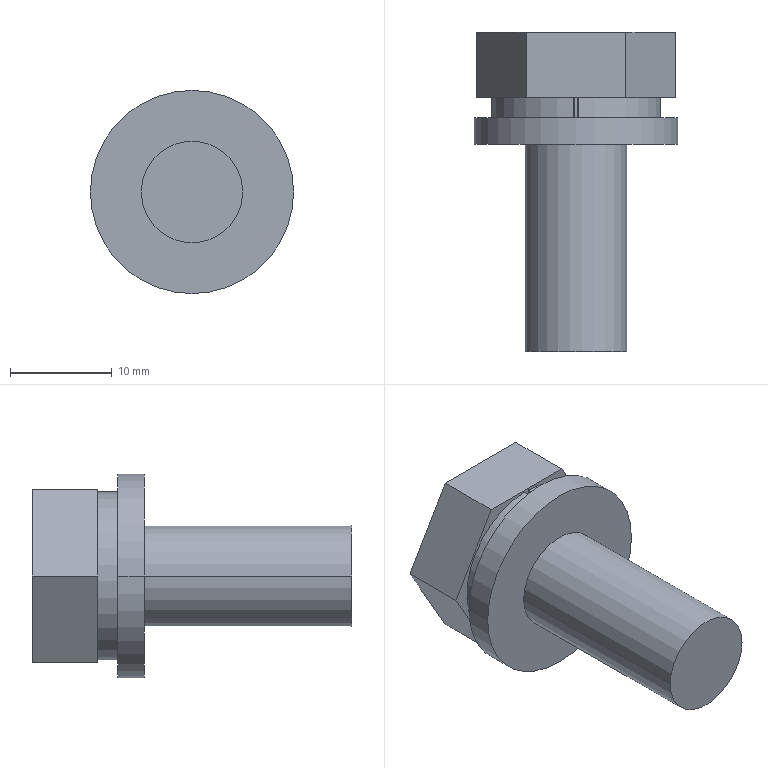Part | STEP file | LIB_68310857_M10X25 | 1 solid | 19 faces | box 20 x 31.4 x 20 mm | volume 4451 mm3 | plane 13 | cylinder 6 | commonest cylinder face diameters 10 x3 20 x2 16.6 x1
STEP:
#1=CARTESIAN_POINT('',(0.,0.,0.));
#2=DIRECTION('',(0.,0.,1.));
#3=DIRECTION('',(1.,0.,0.));
#4=AXIS2_PLACEMENT_3D('',#1,#2,#3);
#5=CARTESIAN_POINT('',(-4.907,0.,-8.5));
#6=VERTEX_POINT('',#5);
#7=CARTESIAN_POINT('',(-9.815,0.,0.));
#8=VERTEX_POINT('',#7);
#9=CARTESIAN_POINT('',(-4.907,0.,-8.5));
#10=DIRECTION('',(-0.5,0.,0.866));
#11=VECTOR('',#10,1.);
#12=LINE('',#9,#11);
#13=CARTESIAN_POINT('',(0.,0.,0.));
#14=DIRECTION('',(0.,1.,0.));
#15=DIRECTION('',(1.,0.,0.));
#16=AXIS2_PLACEMENT_3D('',#13,#14,#15);
#17=PLANE('',#16);
#18=CARTESIAN_POINT('',(-4.907,8.5));
#19=DIRECTION('',(-0.5,-0.866));
#20=VECTOR('',#19,1.);
#21=LINE('',#18,#20);
#22=(GEOMETRIC_REPRESENTATION_CONTEXT(2)PARAMETRIC_REPRESENTATION_CONTEXT()REPRESENTATION_CONTEXT('',''));
#23=DEFINITIONAL_REPRESENTATION('',(#21),#22);
#24=PCURVE('',#17,#23);
#25=CARTESIAN_POINT('',(-4.907,0.,-8.5));
#26=DIRECTION('',(-0.866,0.,-0.5));
#27=DIRECTION('',(-0.5,0.,0.866));
#28=AXIS2_PLACEMENT_3D('',#25,#26,#27);
#29=PLANE('',#28);
#30=CARTESIAN_POINT('',(0.,0.));
#31=DIRECTION('',(1.,0.));
#32=VECTOR('',#31,1.);
#33=LINE('',#30,#32);
#34=(GEOMETRIC_REPRESENTATION_CONTEXT(2)PARAMETRIC_REPRESENTATION_CONTEXT()REPRESENTATION_CONTEXT('',''));
#35=DEFINITIONAL_REPRESENTATION('',(#33),#34);
#36=PCURVE('',#29,#35);
#37=SURFACE_CURVE('',#12,(#24,#36),.PCURVE_S1.);
#38=EDGE_CURVE('',#6,#8,#37,.T.);
#39=ORIENTED_EDGE('',*,*,#38,.T.);
#40=CARTESIAN_POINT('',(-4.907,0.,8.5));
#41=VERTEX_POINT('',#40);
#42=CARTESIAN_POINT('',(-9.815,0.,0.));
#43=DIRECTION('',(0.5,0.,0.866));
#44=VECTOR('',#43,1.);
#45=LINE('',#42,#44);
#46=CARTESIAN_POINT('',(-9.815,0.));
#47=DIRECTION('',(0.5,-0.866));
#48=VECTOR('',#47,1.);
#49=LINE('',#46,#48);
#50=(GEOMETRIC_REPRESENTATION_CONTEXT(2)PARAMETRIC_REPRESENTATION_CONTEXT()REPRESENTATION_CONTEXT('',''));
#51=DEFINITIONAL_REPRESENTATION('',(#49),#50);
#52=PCURVE('',#17,#51);
#53=CARTESIAN_POINT('',(-9.815,0.,0.));
#54=DIRECTION('',(-0.866,0.,0.5));
#55=DIRECTION('',(0.5,0.,0.866));
#56=AXIS2_PLACEMENT_3D('',#53,#54,#55);
#57=PLANE('',#56);
#58=CARTESIAN_POINT('',(0.,0.));
#59=DIRECTION('',(1.,0.));
#60=VECTOR('',#59,1.);
#61=LINE('',#58,#60);
#62=(GEOMETRIC_REPRESENTATION_CONTEXT(2)PARAMETRIC_REPRESENTATION_CONTEXT()REPRESENTATION_CONTEXT('',''));
#63=DEFINITIONAL_REPRESENTATION('',(#61),#62);
#64=PCURVE('',#57,#63);
#65=SURFACE_CURVE('',#45,(#52,#64),.PCURVE_S1.);
#66=EDGE_CURVE('',#8,#41,#65,.T.);
#67=ORIENTED_EDGE('',*,*,#66,.T.);
#68=CARTESIAN_POINT('',(4.907,0.,8.5));
#69=VERTEX_POINT('',#68);
#70=CARTESIAN_POINT('',(-4.907,0.,8.5));
#71=DIRECTION('',(1.,0.,0.));
#72=VECTOR('',#71,1.);
#73=LINE('',#70,#72);
#74=CARTESIAN_POINT('',(-4.907,-8.5));
#75=DIRECTION('',(1.,0.));
#76=VECTOR('',#75,1.);
#77=LINE('',#74,#76);
#78=(GEOMETRIC_REPRESENTATION_CONTEXT(2)PARAMETRIC_REPRESENTATION_CONTEXT()REPRESENTATION_CONTEXT('',''));
#79=DEFINITIONAL_REPRESENTATION('',(#77),#78);
#80=PCURVE('',#17,#79);
#81=CARTESIAN_POINT('',(-4.907,0.,8.5));
#82=DIRECTION('',(0.,0.,1.));
#83=DIRECTION('',(1.,0.,0.));
#84=AXIS2_PLACEMENT_3D('',#81,#82,#83);
#85=PLANE('',#84);
#86=CARTESIAN_POINT('',(0.,0.));
#87=DIRECTION('',(1.,0.));
#88=VECTOR('',#87,1.);
#89=LINE('',#86,#88);
#90=(GEOMETRIC_REPRESENTATION_CONTEXT(2)PARAMETRIC_REPRESENTATION_CONTEXT()REPRESENTATION_CONTEXT('',''));
#91=DEFINITIONAL_REPRESENTATION('',(#89),#90);
#92=PCURVE('',#85,#91);
#93=SURFACE_CURVE('',#73,(#80,#92),.PCURVE_S1.);
#94=EDGE_CURVE('',#41,#69,#93,.T.);
#95=ORIENTED_EDGE('',*,*,#94,.T.);
#96=CARTESIAN_POINT('',(9.815,0.,0.));
#97=VERTEX_POINT('',#96);
#98=CARTESIAN_POINT('',(4.907,0.,8.5));
#99=DIRECTION('',(0.5,0.,-0.866));
#100=VECTOR('',#99,1.);
#101=LINE('',#98,#100);
#102=CARTESIAN_POINT('',(4.907,-8.5));
#103=DIRECTION('',(0.5,0.866));
#104=VECTOR('',#103,1.);
#105=LINE('',#102,#104);
#106=(GEOMETRIC_REPRESENTATION_CONTEXT(2)PARAMETRIC_REPRESENTATION_CONTEXT()REPRESENTATION_CONTEXT('',''));
#107=DEFINITIONAL_REPRESENTATION('',(#105),#106);
#108=PCURVE('',#17,#107);
#109=CARTESIAN_POINT('',(4.907,0.,8.5));
#110=DIRECTION('',(0.866,0.,0.5));
#111=DIRECTION('',(0.5,0.,-0.866));
#112=AXIS2_PLACEMENT_3D('',#109,#110,#111);
#113=PLANE('',#112);
#114=CARTESIAN_POINT('',(0.,0.));
#115=DIRECTION('',(1.,0.));
#116=VECTOR('',#115,1.);
#117=LINE('',#114,#116);
#118=(GEOMETRIC_REPRESENTATION_CONTEXT(2)PARAMETRIC_REPRESENTATION_CONTEXT()REPRESENTATION_CONTEXT('',''));
#119=DEFINITIONAL_REPRESENTATION('',(#117),#118);
#120=PCURVE('',#113,#119);
#121=SURFACE_CURVE('',#101,(#108,#120),.PCURVE_S1.);
#122=EDGE_CURVE('',#69,#97,#121,.T.);
#123=ORIENTED_EDGE('',*,*,#122,.T.);
#124=CARTESIAN_POINT('',(4.907,0.,-8.5));
#125=VERTEX_POINT('',#124);
#126=CARTESIAN_POINT('',(9.815,0.,0.));
#127=DIRECTION('',(-0.5,0.,-0.866));
#128=VECTOR('',#127,1.);
#129=LINE('',#126,#128);
#130=CARTESIAN_POINT('',(9.815,0.));
#131=DIRECTION('',(-0.5,0.866));
#132=VECTOR('',#131,1.);
#133=LINE('',#130,#132);
#134=(GEOMETRIC_REPRESENTATION_CONTEXT(2)PARAMETRIC_REPRESENTATION_CONTEXT()REPRESENTATION_CONTEXT('',''));
#135=DEFINITIONAL_REPRESENTATION('',(#133),#134);
#136=PCURVE('',#17,#135);
#137=CARTESIAN_POINT('',(9.815,0.,0.));
#138=DIRECTION('',(0.866,0.,-0.5));
#139=DIRECTION('',(-0.5,0.,-0.866));
#140=AXIS2_PLACEMENT_3D('',#137,#138,#139);
#141=PLANE('',#140);
#142=CARTESIAN_POINT('',(0.,0.));
#143=DIRECTION('',(1.,0.));
#144=VECTOR('',#143,1.);
#145=LINE('',#142,#144);
#146=(GEOMETRIC_REPRESENTATION_CONTEXT(2)PARAMETRIC_REPRESENTATION_CONTEXT()REPRESENTATION_CONTEXT('',''));
#147=DEFINITIONAL_REPRESENTATION('',(#145),#146);
#148=PCURVE('',#141,#147);
#149=SURFACE_CURVE('',#129,(#136,#148),.PCURVE_S1.);
#150=EDGE_CURVE('',#97,#125,#149,.T.);
#151=ORIENTED_EDGE('',*,*,#150,.T.);
#152=CARTESIAN_POINT('',(4.907,0.,-8.5));
#153=DIRECTION('',(-1.,0.,0.));
#154=VECTOR('',#153,1.);
#155=LINE('',#152,#154);
#156=CARTESIAN_POINT('',(4.907,8.5));
#157=DIRECTION('',(-1.,0.));
#158=VECTOR('',#157,1.);
#159=LINE('',#156,#158);
#160=(GEOMETRIC_REPRESENTATION_CONTEXT(2)PARAMETRIC_REPRESENTATION_CONTEXT()REPRESENTATION_CONTEXT('',''));
#161=DEFINITIONAL_REPRESENTATION('',(#159),#160);
#162=PCURVE('',#17,#161);
#163=CARTESIAN_POINT('',(4.907,0.,-8.5));
#164=DIRECTION('',(0.,0.,-1.));
#165=DIRECTION('',(-1.,0.,0.));
#166=AXIS2_PLACEMENT_3D('',#163,#164,#165);
#167=PLANE('',#166);
#168=CARTESIAN_POINT('',(0.,0.));
#169=DIRECTION('',(1.,0.));
#170=VECTOR('',#169,1.);
#171=LINE('',#168,#170);
#172=(GEOMETRIC_REPRESENTATION_CONTEXT(2)PARAMETRIC_REPRESENTATION_CONTEXT()REPRESENTATION_CONTEXT('',''));
#173=DEFINITIONAL_REPRESENTATION('',(#171),#172);
#174=PCURVE('',#167,#173);
#175=SURFACE_CURVE('',#155,(#162,#174),.PCURVE_S1.);
#176=EDGE_CURVE('',#125,#6,#175,.T.);
#177=ORIENTED_EDGE('',*,*,#176,.T.);
#178=EDGE_LOOP('',(#39,#67,#95,#123,#151,#177));
#179=FACE_BOUND('',#178,.F.);
#180=CARTESIAN_POINT('',(-0.25,0.,8.296));
#181=VERTEX_POINT('',#180);
#182=CARTESIAN_POINT('',(0.25,0.,8.296));
#183=VERTEX_POINT('',#182);
#184=CARTESIAN_POINT('',(0.,0.,0.));
#185=DIRECTION('',(0.,-1.,0.));
#186=DIRECTION('',(-0.03012,0.,0.9995));
#187=AXIS2_PLACEMENT_3D('',#184,#185,#186);
#188=CIRCLE('',#187,8.3);
#189=CARTESIAN_POINT('',(-0.25,-8.296));
#190=CARTESIAN_POINT('',(-14.619,-7.863));
#191=CARTESIAN_POINT('',(-7.06,4.365));
#192=CARTESIAN_POINT('',(0.5,16.592));
#193=CARTESIAN_POINT('',(7.31,3.932));
#194=CARTESIAN_POINT('',(14.119,-8.729));
#195=CARTESIAN_POINT('',(-0.25,-8.296));
#196=(BOUNDED_CURVE()B_SPLINE_CURVE(2,(#189,#190,#191,#192,#193,#194,#195),.UNSPECIFIED.,.T.,.F.)B_SPLINE_CURVE_WITH_KNOTS((1,2,2,2,2,1),(-2.094,0.,2.094,4.189,6.283,8.378),.UNSPECIFIED.)CURVE()GEOMETRIC_REPRESENTATION_ITEM()RATIONAL_B_SPLINE_CURVE((1.,0.5,1.,0.5,1.,0.5,1.))REPRESENTATION_ITEM(''));
#197=(GEOMETRIC_REPRESENTATION_CONTEXT(2)PARAMETRIC_REPRESENTATION_CONTEXT()REPRESENTATION_CONTEXT('',''));
#198=DEFINITIONAL_REPRESENTATION('',(#196),#197);
#199=PCURVE('',#17,#198);
#200=CARTESIAN_POINT('',(0.,0.,0.));
#201=DIRECTION('',(0.,-1.,0.));
#202=DIRECTION('',(0.,0.,-1.));
#203=AXIS2_PLACEMENT_3D('',#200,#201,#202);
#204=CYLINDRICAL_SURFACE('',#203,8.3);
#205=CARTESIAN_POINT('',(3.172,0.));
#206=DIRECTION('',(1.,0.));
#207=VECTOR('',#206,1.);
#208=LINE('',#205,#207);
#209=(GEOMETRIC_REPRESENTATION_CONTEXT(2)PARAMETRIC_REPRESENTATION_CONTEXT()REPRESENTATION_CONTEXT('',''));
#210=DEFINITIONAL_REPRESENTATION('',(#208),#209);
#211=PCURVE('',#204,#210);
#212=SURFACE_CURVE('',#188,(#199,#211),.PCURVE_S1.);
#213=EDGE_CURVE('',#181,#183,#212,.T.);
#214=ORIENTED_EDGE('',*,*,#213,.T.);
#215=CARTESIAN_POINT('',(0.1506,0.,4.998));
#216=VERTEX_POINT('',#215);
#217=CARTESIAN_POINT('',(0.25,0.,8.296));
#218=DIRECTION('',(-0.03012,0.,-0.9995));
#219=VECTOR('',#218,1.);
#220=LINE('',#217,#219);
#221=CARTESIAN_POINT('',(0.25,-8.296));
#222=DIRECTION('',(-0.03012,0.9995));
#223=VECTOR('',#222,1.);
#224=LINE('',#221,#223);
#225=(GEOMETRIC_REPRESENTATION_CONTEXT(2)PARAMETRIC_REPRESENTATION_CONTEXT()REPRESENTATION_CONTEXT('',''));
#226=DEFINITIONAL_REPRESENTATION('',(#224),#225);
#227=PCURVE('',#17,#226);
#228=CARTESIAN_POINT('',(0.25,0.,8.296));
#229=DIRECTION('',(-0.9995,0.,0.03012));
#230=DIRECTION('',(-0.03012,0.,-0.9995));
#231=AXIS2_PLACEMENT_3D('',#228,#229,#230);
#232=PLANE('',#231);
#233=CARTESIAN_POINT('',(0.,0.));
#234=DIRECTION('',(1.,0.));
#235=VECTOR('',#234,1.);
#236=LINE('',#233,#235);
#237=(GEOMETRIC_REPRESENTATION_CONTEXT(2)PARAMETRIC_REPRESENTATION_CONTEXT()REPRESENTATION_CONTEXT('',''));
#238=DEFINITIONAL_REPRESENTATION('',(#236),#237);
#239=PCURVE('',#232,#238);
#240=SURFACE_CURVE('',#220,(#227,#239),.PCURVE_S1.);
#241=EDGE_CURVE('',#183,#216,#240,.T.);
#242=ORIENTED_EDGE('',*,*,#241,.T.);
#243=CARTESIAN_POINT('',(-0.1506,0.,4.998));
#244=VERTEX_POINT('',#243);
#245=CARTESIAN_POINT('',(0.,0.,0.));
#246=DIRECTION('',(0.,-1.,0.));
#247=DIRECTION('',(0.03012,0.,0.9995));
#248=AXIS2_PLACEMENT_3D('',#245,#246,#247);
#249=CIRCLE('',#248,5.);
#250=CARTESIAN_POINT('',(0.1506,-4.998));
#251=CARTESIAN_POINT('',(-8.506,-5.259));
#252=CARTESIAN_POINT('',(-4.403,2.368));
#253=CARTESIAN_POINT('',(-0.3012,9.995));
#254=CARTESIAN_POINT('',(4.253,2.629));
#255=CARTESIAN_POINT('',(8.807,-4.737));
#256=CARTESIAN_POINT('',(0.1506,-4.998));
#257=(BOUNDED_CURVE()B_SPLINE_CURVE(2,(#250,#251,#252,#253,#254,#255,#256),.UNSPECIFIED.,.T.,.F.)B_SPLINE_CURVE_WITH_KNOTS((1,2,2,2,2,1),(-2.094,0.,2.094,4.189,6.283,8.378),.UNSPECIFIED.)CURVE()GEOMETRIC_REPRESENTATION_ITEM()RATIONAL_B_SPLINE_CURVE((1.,0.5,1.,0.5,1.,0.5,1.))REPRESENTATION_ITEM(''));
#258=(GEOMETRIC_REPRESENTATION_CONTEXT(2)PARAMETRIC_REPRESENTATION_CONTEXT()REPRESENTATION_CONTEXT('',''));
#259=DEFINITIONAL_REPRESENTATION('',(#257),#258);
#260=PCURVE('',#17,#259);
#261=CARTESIAN_POINT('',(0.,0.,0.));
#262=DIRECTION('',(0.,-1.,0.));
#263=DIRECTION('',(1.,0.,0.));
#264=AXIS2_PLACEMENT_3D('',#261,#262,#263);
#265=CYLINDRICAL_SURFACE('',#264,5.);
#266=CARTESIAN_POINT('',(1.541,0.));
#267=DIRECTION('',(1.,0.));
#268=VECTOR('',#267,1.);
#269=LINE('',#266,#268);
#270=(GEOMETRIC_REPRESENTATION_CONTEXT(2)PARAMETRIC_REPRESENTATION_CONTEXT()REPRESENTATION_CONTEXT('',''));
#271=DEFINITIONAL_REPRESENTATION('',(#269),#270);
#272=PCURVE('',#265,#271);
#273=SURFACE_CURVE('',#249,(#260,#272),.PCURVE_S1.);
#274=EDGE_CURVE('',#216,#244,#273,.T.);
#275=ORIENTED_EDGE('',*,*,#274,.T.);
#276=CARTESIAN_POINT('',(-0.1506,0.,4.998));
#277=DIRECTION('',(-0.03012,0.,0.9995));
#278=VECTOR('',#277,1.);
#279=LINE('',#276,#278);
#280=CARTESIAN_POINT('',(-0.1506,-4.998));
#281=DIRECTION('',(-0.03012,-0.9995));
#282=VECTOR('',#281,1.);
#283=LINE('',#280,#282);
#284=(GEOMETRIC_REPRESENTATION_CONTEXT(2)PARAMETRIC_REPRESENTATION_CONTEXT()REPRESENTATION_CONTEXT('',''));
#285=DEFINITIONAL_REPRESENTATION('',(#283),#284);
#286=PCURVE('',#17,#285);
#287=CARTESIAN_POINT('',(-0.1506,0.,4.998));
#288=DIRECTION('',(0.9995,0.,0.03012));
#289=DIRECTION('',(-0.03012,0.,0.9995));
#290=AXIS2_PLACEMENT_3D('',#287,#288,#289);
#291=PLANE('',#290);
#292=CARTESIAN_POINT('',(0.,0.));
#293=DIRECTION('',(1.,0.));
#294=VECTOR('',#293,1.);
#295=LINE('',#292,#294);
#296=(GEOMETRIC_REPRESENTATION_CONTEXT(2)PARAMETRIC_REPRESENTATION_CONTEXT()REPRESENTATION_CONTEXT('',''));
#297=DEFINITIONAL_REPRESENTATION('',(#295),#296);
#298=PCURVE('',#291,#297);
#299=SURFACE_CURVE('',#279,(#286,#298),.PCURVE_S1.);
#300=EDGE_CURVE('',#244,#181,#299,.T.);
#301=ORIENTED_EDGE('',*,*,#300,.T.);
#302=EDGE_LOOP('',(#214,#242,#275,#301));
#303=FACE_BOUND('',#302,.F.);
#304=ADVANCED_FACE('',(#179,#303),#17,.F.);
#305=ORIENTED_EDGE('',*,*,#38,.F.);
#306=CARTESIAN_POINT('',(-4.907,6.4,-8.5));
#307=VERTEX_POINT('',#306);
#308=CARTESIAN_POINT('',(-4.907,0.,-8.5));
#309=DIRECTION('',(0.,1.,0.));
#310=VECTOR('',#309,1.);
#311=LINE('',#308,#310);
#312=CARTESIAN_POINT('',(0.,0.));
#313=DIRECTION('',(0.,1.));
#314=VECTOR('',#313,1.);
#315=LINE('',#312,#314);
#316=(GEOMETRIC_REPRESENTATION_CONTEXT(2)PARAMETRIC_REPRESENTATION_CONTEXT()REPRESENTATION_CONTEXT('',''));
#317=DEFINITIONAL_REPRESENTATION('',(#315),#316);
#318=PCURVE('',#29,#317);
#319=CARTESIAN_POINT('',(9.815,0.));
#320=DIRECTION('',(0.,1.));
#321=VECTOR('',#320,1.);
#322=LINE('',#319,#321);
#323=(GEOMETRIC_REPRESENTATION_CONTEXT(2)PARAMETRIC_REPRESENTATION_CONTEXT()REPRESENTATION_CONTEXT('',''));
#324=DEFINITIONAL_REPRESENTATION('',(#322),#323);
#325=PCURVE('',#167,#324);
#326=SURFACE_CURVE('',#311,(#318,#325),.PCURVE_S1.);
#327=EDGE_CURVE('',#6,#307,#326,.T.);
#328=ORIENTED_EDGE('',*,*,#327,.T.);
#329=CARTESIAN_POINT('',(-9.815,6.4,0.));
#330=VERTEX_POINT('',#329);
#331=CARTESIAN_POINT('',(-4.907,6.4,-8.5));
#332=DIRECTION('',(-0.5,0.,0.866));
#333=VECTOR('',#332,1.);
#334=LINE('',#331,#333);
#335=CARTESIAN_POINT('',(0.,6.4));
#336=DIRECTION('',(1.,0.));
#337=VECTOR('',#336,1.);
#338=LINE('',#335,#337);
#339=(GEOMETRIC_REPRESENTATION_CONTEXT(2)PARAMETRIC_REPRESENTATION_CONTEXT()REPRESENTATION_CONTEXT('',''));
#340=DEFINITIONAL_REPRESENTATION('',(#338),#339);
#341=PCURVE('',#29,#340);
#342=CARTESIAN_POINT('',(0.,6.4,0.));
#343=DIRECTION('',(0.,1.,0.));
#344=DIRECTION('',(1.,0.,0.));
#345=AXIS2_PLACEMENT_3D('',#342,#343,#344);
#346=PLANE('',#345);
#347=CARTESIAN_POINT('',(-4.907,8.5));
#348=DIRECTION('',(-0.5,-0.866));
#349=VECTOR('',#348,1.);
#350=LINE('',#347,#349);
#351=(GEOMETRIC_REPRESENTATION_CONTEXT(2)PARAMETRIC_REPRESENTATION_CONTEXT()REPRESENTATION_CONTEXT('',''));
#352=DEFINITIONAL_REPRESENTATION('',(#350),#351);
#353=PCURVE('',#346,#352);
#354=SURFACE_CURVE('',#334,(#341,#353),.PCURVE_S1.);
#355=EDGE_CURVE('',#307,#330,#354,.T.);
#356=ORIENTED_EDGE('',*,*,#355,.T.);
#357=CARTESIAN_POINT('',(-9.815,0.,0.));
#358=DIRECTION('',(0.,1.,0.));
#359=VECTOR('',#358,1.);
#360=LINE('',#357,#359);
#361=CARTESIAN_POINT('',(9.815,0.));
#362=DIRECTION('',(0.,1.));
#363=VECTOR('',#362,1.);
#364=LINE('',#361,#363);
#365=(GEOMETRIC_REPRESENTATION_CONTEXT(2)PARAMETRIC_REPRESENTATION_CONTEXT()REPRESENTATION_CONTEXT('',''));
#366=DEFINITIONAL_REPRESENTATION('',(#364),#365);
#367=PCURVE('',#29,#366);
#368=CARTESIAN_POINT('',(0.,0.));
#369=DIRECTION('',(0.,1.));
#370=VECTOR('',#369,1.);
#371=LINE('',#368,#370);
#372=(GEOMETRIC_REPRESENTATION_CONTEXT(2)PARAMETRIC_REPRESENTATION_CONTEXT()REPRESENTATION_CONTEXT('',''));
#373=DEFINITIONAL_REPRESENTATION('',(#371),#372);
#374=PCURVE('',#57,#373);
#375=SURFACE_CURVE('',#360,(#367,#374),.PCURVE_S1.);
#376=EDGE_CURVE('',#8,#330,#375,.T.);
#377=ORIENTED_EDGE('',*,*,#376,.F.);
#378=EDGE_LOOP('',(#305,#328,#356,#377));
#379=FACE_BOUND('',#378,.F.);
#380=ADVANCED_FACE('',(#379),#29,.T.);
#381=ORIENTED_EDGE('',*,*,#176,.F.);
#382=CARTESIAN_POINT('',(4.907,6.4,-8.5));
#383=VERTEX_POINT('',#382);
#384=CARTESIAN_POINT('',(4.907,0.,-8.5));
#385=DIRECTION('',(0.,1.,0.));
#386=VECTOR('',#385,1.);
#387=LINE('',#384,#386);
#388=CARTESIAN_POINT('',(0.,0.));
#389=DIRECTION('',(0.,1.));
#390=VECTOR('',#389,1.);
#391=LINE('',#388,#390);
#392=(GEOMETRIC_REPRESENTATION_CONTEXT(2)PARAMETRIC_REPRESENTATION_CONTEXT()REPRESENTATION_CONTEXT('',''));
#393=DEFINITIONAL_REPRESENTATION('',(#391),#392);
#394=PCURVE('',#167,#393);
#395=CARTESIAN_POINT('',(9.815,0.));
#396=DIRECTION('',(0.,1.));
#397=VECTOR('',#396,1.);
#398=LINE('',#395,#397);
#399=(GEOMETRIC_REPRESENTATION_CONTEXT(2)PARAMETRIC_REPRESENTATION_CONTEXT()REPRESENTATION_CONTEXT('',''));
#400=DEFINITIONAL_REPRESENTATION('',(#398),#399);
#401=PCURVE('',#141,#400);
#402=SURFACE_CURVE('',#387,(#394,#401),.PCURVE_S1.);
#403=EDGE_CURVE('',#125,#383,#402,.T.);
#404=ORIENTED_EDGE('',*,*,#403,.T.);
#405=CARTESIAN_POINT('',(4.907,6.4,-8.5));
#406=DIRECTION('',(-1.,0.,0.));
#407=VECTOR('',#406,1.);
#408=LINE('',#405,#407);
#409=CARTESIAN_POINT('',(0.,6.4));
#410=DIRECTION('',(1.,0.));
#411=VECTOR('',#410,1.);
#412=LINE('',#409,#411);
#413=(GEOMETRIC_REPRESENTATION_CONTEXT(2)PARAMETRIC_REPRESENTATION_CONTEXT()REPRESENTATION_CONTEXT('',''));
#414=DEFINITIONAL_REPRESENTATION('',(#412),#413);
#415=PCURVE('',#167,#414);
#416=CARTESIAN_POINT('',(4.907,8.5));
#417=DIRECTION('',(-1.,0.));
#418=VECTOR('',#417,1.);
#419=LINE('',#416,#418);
#420=(GEOMETRIC_REPRESENTATION_CONTEXT(2)PARAMETRIC_REPRESENTATION_CONTEXT()REPRESENTATION_CONTEXT('',''));
#421=DEFINITIONAL_REPRESENTATION('',(#419),#420);
#422=PCURVE('',#346,#421);
#423=SURFACE_CURVE('',#408,(#415,#422),.PCURVE_S1.);
#424=EDGE_CURVE('',#383,#307,#423,.T.);
#425=ORIENTED_EDGE('',*,*,#424,.T.);
#426=ORIENTED_EDGE('',*,*,#327,.F.);
#427=EDGE_LOOP('',(#381,#404,#425,#426));
#428=FACE_BOUND('',#427,.F.);
#429=ADVANCED_FACE('',(#428),#167,.T.);
#430=ORIENTED_EDGE('',*,*,#150,.F.);
#431=CARTESIAN_POINT('',(9.815,6.4,0.));
#432=VERTEX_POINT('',#431);
#433=CARTESIAN_POINT('',(9.815,0.,0.));
#434=DIRECTION('',(0.,1.,0.));
#435=VECTOR('',#434,1.);
#436=LINE('',#433,#435);
#437=CARTESIAN_POINT('',(0.,0.));
#438=DIRECTION('',(0.,1.));
#439=VECTOR('',#438,1.);
#440=LINE('',#437,#439);
#441=(GEOMETRIC_REPRESENTATION_CONTEXT(2)PARAMETRIC_REPRESENTATION_CONTEXT()REPRESENTATION_CONTEXT('',''));
#442=DEFINITIONAL_REPRESENTATION('',(#440),#441);
#443=PCURVE('',#141,#442);
#444=CARTESIAN_POINT('',(9.815,0.));
#445=DIRECTION('',(0.,1.));
#446=VECTOR('',#445,1.);
#447=LINE('',#444,#446);
#448=(GEOMETRIC_REPRESENTATION_CONTEXT(2)PARAMETRIC_REPRESENTATION_CONTEXT()REPRESENTATION_CONTEXT('',''));
#449=DEFINITIONAL_REPRESENTATION('',(#447),#448);
#450=PCURVE('',#113,#449);
#451=SURFACE_CURVE('',#436,(#443,#450),.PCURVE_S1.);
#452=EDGE_CURVE('',#97,#432,#451,.T.);
#453=ORIENTED_EDGE('',*,*,#452,.T.);
#454=CARTESIAN_POINT('',(9.815,6.4,0.));
#455=DIRECTION('',(-0.5,0.,-0.866));
#456=VECTOR('',#455,1.);
#457=LINE('',#454,#456);
#458=CARTESIAN_POINT('',(0.,6.4));
#459=DIRECTION('',(1.,0.));
#460=VECTOR('',#459,1.);
#461=LINE('',#458,#460);
#462=(GEOMETRIC_REPRESENTATION_CONTEXT(2)PARAMETRIC_REPRESENTATION_CONTEXT()REPRESENTATION_CONTEXT('',''));
#463=DEFINITIONAL_REPRESENTATION('',(#461),#462);
#464=PCURVE('',#141,#463);
#465=CARTESIAN_POINT('',(9.815,0.));
#466=DIRECTION('',(-0.5,0.866));
#467=VECTOR('',#466,1.);
#468=LINE('',#465,#467);
#469=(GEOMETRIC_REPRESENTATION_CONTEXT(2)PARAMETRIC_REPRESENTATION_CONTEXT()REPRESENTATION_CONTEXT('',''));
#470=DEFINITIONAL_REPRESENTATION('',(#468),#469);
#471=PCURVE('',#346,#470);
#472=SURFACE_CURVE('',#457,(#464,#471),.PCURVE_S1.);
#473=EDGE_CURVE('',#432,#383,#472,.T.);
#474=ORIENTED_EDGE('',*,*,#473,.T.);
#475=ORIENTED_EDGE('',*,*,#403,.F.);
#476=EDGE_LOOP('',(#430,#453,#474,#475));
#477=FACE_BOUND('',#476,.F.);
#478=ADVANCED_FACE('',(#477),#141,.T.);
#479=ORIENTED_EDGE('',*,*,#122,.F.);
#480=CARTESIAN_POINT('',(4.907,6.4,8.5));
#481=VERTEX_POINT('',#480);
#482=CARTESIAN_POINT('',(4.907,0.,8.5));
#483=DIRECTION('',(0.,1.,0.));
#484=VECTOR('',#483,1.);
#485=LINE('',#482,#484);
#486=CARTESIAN_POINT('',(0.,0.));
#487=DIRECTION('',(0.,1.));
#488=VECTOR('',#487,1.);
#489=LINE('',#486,#488);
#490=(GEOMETRIC_REPRESENTATION_CONTEXT(2)PARAMETRIC_REPRESENTATION_CONTEXT()REPRESENTATION_CONTEXT('',''));
#491=DEFINITIONAL_REPRESENTATION('',(#489),#490);
#492=PCURVE('',#113,#491);
#493=CARTESIAN_POINT('',(9.815,0.));
#494=DIRECTION('',(0.,1.));
#495=VECTOR('',#494,1.);
#496=LINE('',#493,#495);
#497=(GEOMETRIC_REPRESENTATION_CONTEXT(2)PARAMETRIC_REPRESENTATION_CONTEXT()REPRESENTATION_CONTEXT('',''));
#498=DEFINITIONAL_REPRESENTATION('',(#496),#497);
#499=PCURVE('',#85,#498);
#500=SURFACE_CURVE('',#485,(#492,#499),.PCURVE_S1.);
#501=EDGE_CURVE('',#69,#481,#500,.T.);
#502=ORIENTED_EDGE('',*,*,#501,.T.);
#503=CARTESIAN_POINT('',(4.907,6.4,8.5));
#504=DIRECTION('',(0.5,0.,-0.866));
#505=VECTOR('',#504,1.);
#506=LINE('',#503,#505);
#507=CARTESIAN_POINT('',(0.,6.4));
#508=DIRECTION('',(1.,0.));
#509=VECTOR('',#508,1.);
#510=LINE('',#507,#509);
#511=(GEOMETRIC_REPRESENTATION_CONTEXT(2)PARAMETRIC_REPRESENTATION_CONTEXT()REPRESENTATION_CONTEXT('',''));
#512=DEFINITIONAL_REPRESENTATION('',(#510),#511);
#513=PCURVE('',#113,#512);
#514=CARTESIAN_POINT('',(4.907,-8.5));
#515=DIRECTION('',(0.5,0.866));
#516=VECTOR('',#515,1.);
#517=LINE('',#514,#516);
#518=(GEOMETRIC_REPRESENTATION_CONTEXT(2)PARAMETRIC_REPRESENTATION_CONTEXT()REPRESENTATION_CONTEXT('',''));
#519=DEFINITIONAL_REPRESENTATION('',(#517),#518);
#520=PCURVE('',#346,#519);
#521=SURFACE_CURVE('',#506,(#513,#520),.PCURVE_S1.);
#522=EDGE_CURVE('',#481,#432,#521,.T.);
#523=ORIENTED_EDGE('',*,*,#522,.T.);
#524=ORIENTED_EDGE('',*,*,#452,.F.);
#525=EDGE_LOOP('',(#479,#502,#523,#524));
#526=FACE_BOUND('',#525,.F.);
#527=ADVANCED_FACE('',(#526),#113,.T.);
#528=ORIENTED_EDGE('',*,*,#94,.F.);
#529=CARTESIAN_POINT('',(-4.907,6.4,8.5));
#530=VERTEX_POINT('',#529);
#531=CARTESIAN_POINT('',(-4.907,0.,8.5));
#532=DIRECTION('',(0.,1.,0.));
#533=VECTOR('',#532,1.);
#534=LINE('',#531,#533);
#535=CARTESIAN_POINT('',(0.,0.));
#536=DIRECTION('',(0.,1.));
#537=VECTOR('',#536,1.);
#538=LINE('',#535,#537);
#539=(GEOMETRIC_REPRESENTATION_CONTEXT(2)PARAMETRIC_REPRESENTATION_CONTEXT()REPRESENTATION_CONTEXT('',''));
#540=DEFINITIONAL_REPRESENTATION('',(#538),#539);
#541=PCURVE('',#85,#540);
#542=CARTESIAN_POINT('',(9.815,0.));
#543=DIRECTION('',(0.,1.));
#544=VECTOR('',#543,1.);
#545=LINE('',#542,#544);
#546=(GEOMETRIC_REPRESENTATION_CONTEXT(2)PARAMETRIC_REPRESENTATION_CONTEXT()REPRESENTATION_CONTEXT('',''));
#547=DEFINITIONAL_REPRESENTATION('',(#545),#546);
#548=PCURVE('',#57,#547);
#549=SURFACE_CURVE('',#534,(#541,#548),.PCURVE_S1.);
#550=EDGE_CURVE('',#41,#530,#549,.T.);
#551=ORIENTED_EDGE('',*,*,#550,.T.);
#552=CARTESIAN_POINT('',(-4.907,6.4,8.5));
#553=DIRECTION('',(1.,0.,0.));
#554=VECTOR('',#553,1.);
#555=LINE('',#552,#554);
#556=CARTESIAN_POINT('',(0.,6.4));
#557=DIRECTION('',(1.,0.));
#558=VECTOR('',#557,1.);
#559=LINE('',#556,#558);
#560=(GEOMETRIC_REPRESENTATION_CONTEXT(2)PARAMETRIC_REPRESENTATION_CONTEXT()REPRESENTATION_CONTEXT('',''));
#561=DEFINITIONAL_REPRESENTATION('',(#559),#560);
#562=PCURVE('',#85,#561);
#563=CARTESIAN_POINT('',(-4.907,-8.5));
#564=DIRECTION('',(1.,0.));
#565=VECTOR('',#564,1.);
#566=LINE('',#563,#565);
#567=(GEOMETRIC_REPRESENTATION_CONTEXT(2)PARAMETRIC_REPRESENTATION_CONTEXT()REPRESENTATION_CONTEXT('',''));
#568=DEFINITIONAL_REPRESENTATION('',(#566),#567);
#569=PCURVE('',#346,#568);
#570=SURFACE_CURVE('',#555,(#562,#569),.PCURVE_S1.);
#571=EDGE_CURVE('',#530,#481,#570,.T.);
#572=ORIENTED_EDGE('',*,*,#571,.T.);
#573=ORIENTED_EDGE('',*,*,#501,.F.);
#574=EDGE_LOOP('',(#528,#551,#572,#573));
#575=FACE_BOUND('',#574,.F.);
#576=ADVANCED_FACE('',(#575),#85,.T.);
#577=ORIENTED_EDGE('',*,*,#66,.F.);
#578=ORIENTED_EDGE('',*,*,#376,.T.);
#579=CARTESIAN_POINT('',(-9.815,6.4,0.));
#580=DIRECTION('',(0.5,0.,0.866));
#581=VECTOR('',#580,1.);
#582=LINE('',#579,#581);
#583=CARTESIAN_POINT('',(0.,6.4));
#584=DIRECTION('',(1.,0.));
#585=VECTOR('',#584,1.);
#586=LINE('',#583,#585);
#587=(GEOMETRIC_REPRESENTATION_CONTEXT(2)PARAMETRIC_REPRESENTATION_CONTEXT()REPRESENTATION_CONTEXT('',''));
#588=DEFINITIONAL_REPRESENTATION('',(#586),#587);
#589=PCURVE('',#57,#588);
#590=CARTESIAN_POINT('',(-9.815,0.));
#591=DIRECTION('',(0.5,-0.866));
#592=VECTOR('',#591,1.);
#593=LINE('',#590,#592);
#594=(GEOMETRIC_REPRESENTATION_CONTEXT(2)PARAMETRIC_REPRESENTATION_CONTEXT()REPRESENTATION_CONTEXT('',''));
#595=DEFINITIONAL_REPRESENTATION('',(#593),#594);
#596=PCURVE('',#346,#595);
#597=SURFACE_CURVE('',#582,(#589,#596),.PCURVE_S1.);
#598=EDGE_CURVE('',#330,#530,#597,.T.);
#599=ORIENTED_EDGE('',*,*,#598,.T.);
#600=ORIENTED_EDGE('',*,*,#550,.F.);
#601=EDGE_LOOP('',(#577,#578,#599,#600));
#602=FACE_BOUND('',#601,.F.);
#603=ADVANCED_FACE('',(#602),#57,.T.);
#604=ORIENTED_EDGE('',*,*,#355,.F.);
#605=ORIENTED_EDGE('',*,*,#424,.F.);
#606=ORIENTED_EDGE('',*,*,#473,.F.);
#607=ORIENTED_EDGE('',*,*,#522,.F.);
#608=ORIENTED_EDGE('',*,*,#571,.F.);
#609=ORIENTED_EDGE('',*,*,#598,.F.);
#610=EDGE_LOOP('',(#604,#605,#606,#607,#608,#609));
#611=FACE_BOUND('',#610,.F.);
#612=ADVANCED_FACE('',(#611),#346,.T.);
#613=CARTESIAN_POINT('',(-0.25,-2.,8.296));
#614=VERTEX_POINT('',#613);
#615=CARTESIAN_POINT('',(-0.25,0.,8.296));
#616=DIRECTION('',(0.,-1.,0.));
#617=VECTOR('',#616,1.);
#618=LINE('',#615,#617);
#619=CARTESIAN_POINT('',(3.172,0.));
#620=DIRECTION('',(0.,1.));
#621=VECTOR('',#620,1.);
#622=LINE('',#619,#621);
#623=(GEOMETRIC_REPRESENTATION_CONTEXT(2)PARAMETRIC_REPRESENTATION_CONTEXT()REPRESENTATION_CONTEXT('',''));
#624=DEFINITIONAL_REPRESENTATION('',(#622),#623);
#625=PCURVE('',#204,#624);
#626=CARTESIAN_POINT('',(3.3,0.));
#627=DIRECTION('',(0.,1.));
#628=VECTOR('',#627,1.);
#629=LINE('',#626,#628);
#630=(GEOMETRIC_REPRESENTATION_CONTEXT(2)PARAMETRIC_REPRESENTATION_CONTEXT()REPRESENTATION_CONTEXT('',''));
#631=DEFINITIONAL_REPRESENTATION('',(#629),#630);
#632=PCURVE('',#291,#631);
#633=SURFACE_CURVE('',#618,(#625,#632),.PCURVE_S1.);
#634=EDGE_CURVE('',#181,#614,#633,.T.);
#635=ORIENTED_EDGE('',*,*,#634,.F.);
#636=ORIENTED_EDGE('',*,*,#213,.T.);
#637=CARTESIAN_POINT('',(0.25,-2.,8.296));
#638=VERTEX_POINT('',#637);
#639=CARTESIAN_POINT('',(0.25,0.,8.296));
#640=DIRECTION('',(0.,-1.,0.));
#641=VECTOR('',#640,1.);
#642=LINE('',#639,#641);
#643=CARTESIAN_POINT('',(9.395,0.));
#644=DIRECTION('',(0.,1.));
#645=VECTOR('',#644,1.);
#646=LINE('',#643,#645);
#647=(GEOMETRIC_REPRESENTATION_CONTEXT(2)PARAMETRIC_REPRESENTATION_CONTEXT()REPRESENTATION_CONTEXT('',''));
#648=DEFINITIONAL_REPRESENTATION('',(#646),#647);
#649=PCURVE('',#204,#648);
#650=CARTESIAN_POINT('',(0.,0.));
#651=DIRECTION('',(0.,1.));
#652=VECTOR('',#651,1.);
#653=LINE('',#650,#652);
#654=(GEOMETRIC_REPRESENTATION_CONTEXT(2)PARAMETRIC_REPRESENTATION_CONTEXT()REPRESENTATION_CONTEXT('',''));
#655=DEFINITIONAL_REPRESENTATION('',(#653),#654);
#656=PCURVE('',#232,#655);
#657=SURFACE_CURVE('',#642,(#649,#656),.PCURVE_S1.);
#658=EDGE_CURVE('',#183,#638,#657,.T.);
#659=ORIENTED_EDGE('',*,*,#658,.T.);
#660=CARTESIAN_POINT('',(0.,-2.,0.));
#661=DIRECTION('',(0.,-1.,0.));
#662=DIRECTION('',(-0.03012,0.,0.9995));
#663=AXIS2_PLACEMENT_3D('',#660,#661,#662);
#664=CIRCLE('',#663,8.3);
#665=CARTESIAN_POINT('',(3.172,2.));
#666=DIRECTION('',(1.,0.));
#667=VECTOR('',#666,1.);
#668=LINE('',#665,#667);
#669=(GEOMETRIC_REPRESENTATION_CONTEXT(2)PARAMETRIC_REPRESENTATION_CONTEXT()REPRESENTATION_CONTEXT('',''));
#670=DEFINITIONAL_REPRESENTATION('',(#668),#669);
#671=PCURVE('',#204,#670);
#672=CARTESIAN_POINT('',(0.,-2.,0.));
#673=DIRECTION('',(0.,-1.,0.));
#674=DIRECTION('',(1.,0.,0.));
#675=AXIS2_PLACEMENT_3D('',#672,#673,#674);
#676=PLANE('',#675);
#677=CARTESIAN_POINT('',(0.,0.));
#678=DIRECTION('',(-0.03012,0.9995));
#679=AXIS2_PLACEMENT_2D('',#677,#678);
#680=CIRCLE('',#679,8.3);
#681=(GEOMETRIC_REPRESENTATION_CONTEXT(2)PARAMETRIC_REPRESENTATION_CONTEXT()REPRESENTATION_CONTEXT('',''));
#682=DEFINITIONAL_REPRESENTATION('',(#680),#681);
#683=PCURVE('',#676,#682);
#684=SURFACE_CURVE('',#664,(#671,#683),.PCURVE_S1.);
#685=EDGE_CURVE('',#614,#638,#684,.T.);
#686=ORIENTED_EDGE('',*,*,#685,.F.);
#687=EDGE_LOOP('',(#635,#636,#659,#686));
#688=FACE_BOUND('',#687,.T.);
#689=ADVANCED_FACE('',(#688),#204,.T.);
#690=CARTESIAN_POINT('',(10.,-2.,0.));
#691=VERTEX_POINT('',#690);
#692=CARTESIAN_POINT('',(-10.,-2.,0.));
#693=VERTEX_POINT('',#692);
#694=CARTESIAN_POINT('',(0.,-2.,0.));
#695=DIRECTION('',(0.,-1.,0.));
#696=DIRECTION('',(1.,0.,0.));
#697=AXIS2_PLACEMENT_3D('',#694,#695,#696);
#698=CIRCLE('',#697,10.);
#699=CARTESIAN_POINT('',(0.,0.));
#700=DIRECTION('',(1.,0.));
#701=AXIS2_PLACEMENT_2D('',#699,#700);
#702=CIRCLE('',#701,10.);
#703=(GEOMETRIC_REPRESENTATION_CONTEXT(2)PARAMETRIC_REPRESENTATION_CONTEXT()REPRESENTATION_CONTEXT('',''));
#704=DEFINITIONAL_REPRESENTATION('',(#702),#703);
#705=PCURVE('',#676,#704);
#706=CARTESIAN_POINT('',(0.,-2.,0.));
#707=DIRECTION('',(0.,-1.,0.));
#708=DIRECTION('',(1.,0.,0.));
#709=AXIS2_PLACEMENT_3D('',#706,#707,#708);
#710=CYLINDRICAL_SURFACE('',#709,10.);
#711=CARTESIAN_POINT('',(0.,0.));
#712=DIRECTION('',(1.,0.));
#713=VECTOR('',#712,1.);
#714=LINE('',#711,#713);
#715=(GEOMETRIC_REPRESENTATION_CONTEXT(2)PARAMETRIC_REPRESENTATION_CONTEXT()REPRESENTATION_CONTEXT('',''));
#716=DEFINITIONAL_REPRESENTATION('',(#714),#715);
#717=PCURVE('',#710,#716);
#718=SURFACE_CURVE('',#698,(#705,#717),.PCURVE_S1.);
#719=EDGE_CURVE('',#691,#693,#718,.T.);
#720=ORIENTED_EDGE('',*,*,#719,.T.);
#721=CARTESIAN_POINT('',(0.,-2.,0.));
#722=DIRECTION('',(0.,-1.,0.));
#723=DIRECTION('',(-1.,0.,0.));
#724=AXIS2_PLACEMENT_3D('',#721,#722,#723);
#725=CIRCLE('',#724,10.);
#726=CARTESIAN_POINT('',(0.,0.));
#727=DIRECTION('',(-1.,0.));
#728=AXIS2_PLACEMENT_2D('',#726,#727);
#729=CIRCLE('',#728,10.);
#730=(GEOMETRIC_REPRESENTATION_CONTEXT(2)PARAMETRIC_REPRESENTATION_CONTEXT()REPRESENTATION_CONTEXT('',''));
#731=DEFINITIONAL_REPRESENTATION('',(#729),#730);
#732=PCURVE('',#676,#731);
#733=CARTESIAN_POINT('',(0.,-2.,0.));
#734=DIRECTION('',(0.,-1.,0.));
#735=DIRECTION('',(1.,0.,0.));
#736=AXIS2_PLACEMENT_3D('',#733,#734,#735);
#737=CYLINDRICAL_SURFACE('',#736,10.);
#738=CARTESIAN_POINT('',(3.142,0.));
#739=DIRECTION('',(1.,0.));
#740=VECTOR('',#739,1.);
#741=LINE('',#738,#740);
#742=(GEOMETRIC_REPRESENTATION_CONTEXT(2)PARAMETRIC_REPRESENTATION_CONTEXT()REPRESENTATION_CONTEXT('',''));
#743=DEFINITIONAL_REPRESENTATION('',(#741),#742);
#744=PCURVE('',#737,#743);
#745=SURFACE_CURVE('',#725,(#732,#744),.PCURVE_S1.);
#746=EDGE_CURVE('',#693,#691,#745,.T.);
#747=ORIENTED_EDGE('',*,*,#746,.T.);
#748=EDGE_LOOP('',(#720,#747));
#749=FACE_BOUND('',#748,.F.);
#750=ORIENTED_EDGE('',*,*,#685,.F.);
#751=CARTESIAN_POINT('',(-0.1506,-2.,4.998));
#752=VERTEX_POINT('',#751);
#753=CARTESIAN_POINT('',(-0.1506,-2.,4.998));
#754=DIRECTION('',(-0.03012,0.,0.9995));
#755=VECTOR('',#754,1.);
#756=LINE('',#753,#755);
#757=CARTESIAN_POINT('',(-0.1506,4.998));
#758=DIRECTION('',(-0.03012,0.9995));
#759=VECTOR('',#758,1.);
#760=LINE('',#757,#759);
#761=(GEOMETRIC_REPRESENTATION_CONTEXT(2)PARAMETRIC_REPRESENTATION_CONTEXT()REPRESENTATION_CONTEXT('',''));
#762=DEFINITIONAL_REPRESENTATION('',(#760),#761);
#763=PCURVE('',#676,#762);
#764=CARTESIAN_POINT('',(0.,2.));
#765=DIRECTION('',(1.,0.));
#766=VECTOR('',#765,1.);
#767=LINE('',#764,#766);
#768=(GEOMETRIC_REPRESENTATION_CONTEXT(2)PARAMETRIC_REPRESENTATION_CONTEXT()REPRESENTATION_CONTEXT('',''));
#769=DEFINITIONAL_REPRESENTATION('',(#767),#768);
#770=PCURVE('',#291,#769);
#771=SURFACE_CURVE('',#756,(#763,#770),.PCURVE_S1.);
#772=EDGE_CURVE('',#752,#614,#771,.T.);
#773=ORIENTED_EDGE('',*,*,#772,.F.);
#774=CARTESIAN_POINT('',(0.1506,-2.,4.998));
#775=VERTEX_POINT('',#774);
#776=CARTESIAN_POINT('',(0.,-2.,0.));
#777=DIRECTION('',(0.,-1.,0.));
#778=DIRECTION('',(0.03012,0.,0.9995));
#779=AXIS2_PLACEMENT_3D('',#776,#777,#778);
#780=CIRCLE('',#779,5.);
#781=CARTESIAN_POINT('',(0.,0.));
#782=DIRECTION('',(0.03012,0.9995));
#783=AXIS2_PLACEMENT_2D('',#781,#782);
#784=CIRCLE('',#783,5.);
#785=(GEOMETRIC_REPRESENTATION_CONTEXT(2)PARAMETRIC_REPRESENTATION_CONTEXT()REPRESENTATION_CONTEXT('',''));
#786=DEFINITIONAL_REPRESENTATION('',(#784),#785);
#787=PCURVE('',#676,#786);
#788=CARTESIAN_POINT('',(1.541,2.));
#789=DIRECTION('',(1.,0.));
#790=VECTOR('',#789,1.);
#791=LINE('',#788,#790);
#792=(GEOMETRIC_REPRESENTATION_CONTEXT(2)PARAMETRIC_REPRESENTATION_CONTEXT()REPRESENTATION_CONTEXT('',''));
#793=DEFINITIONAL_REPRESENTATION('',(#791),#792);
#794=PCURVE('',#265,#793);
#795=SURFACE_CURVE('',#780,(#787,#794),.PCURVE_S1.);
#796=EDGE_CURVE('',#775,#752,#795,.T.);
#797=ORIENTED_EDGE('',*,*,#796,.F.);
#798=CARTESIAN_POINT('',(0.25,-2.,8.296));
#799=DIRECTION('',(-0.03012,0.,-0.9995));
#800=VECTOR('',#799,1.);
#801=LINE('',#798,#800);
#802=CARTESIAN_POINT('',(0.25,8.296));
#803=DIRECTION('',(-0.03012,-0.9995));
#804=VECTOR('',#803,1.);
#805=LINE('',#802,#804);
#806=(GEOMETRIC_REPRESENTATION_CONTEXT(2)PARAMETRIC_REPRESENTATION_CONTEXT()REPRESENTATION_CONTEXT('',''));
#807=DEFINITIONAL_REPRESENTATION('',(#805),#806);
#808=PCURVE('',#676,#807);
#809=CARTESIAN_POINT('',(0.,2.));
#810=DIRECTION('',(1.,0.));
#811=VECTOR('',#810,1.);
#812=LINE('',#809,#811);
#813=(GEOMETRIC_REPRESENTATION_CONTEXT(2)PARAMETRIC_REPRESENTATION_CONTEXT()REPRESENTATION_CONTEXT('',''));
#814=DEFINITIONAL_REPRESENTATION('',(#812),#813);
#815=PCURVE('',#232,#814);
#816=SURFACE_CURVE('',#801,(#808,#815),.PCURVE_S1.);
#817=EDGE_CURVE('',#638,#775,#816,.T.);
#818=ORIENTED_EDGE('',*,*,#817,.F.);
#819=EDGE_LOOP('',(#750,#773,#797,#818));
#820=FACE_BOUND('',#819,.F.);
#821=ADVANCED_FACE('',(#749,#820),#676,.F.);
#822=CARTESIAN_POINT('',(-10.,-4.6,0.));
#823=VERTEX_POINT('',#822);
#824=CARTESIAN_POINT('',(-10.,-2.,0.));
#825=DIRECTION('',(0.,-1.,0.));
#826=VECTOR('',#825,1.);
#827=LINE('',#824,#826);
#828=CARTESIAN_POINT('',(3.142,0.));
#829=DIRECTION('',(0.,1.));
#830=VECTOR('',#829,1.);
#831=LINE('',#828,#830);
#832=(GEOMETRIC_REPRESENTATION_CONTEXT(2)PARAMETRIC_REPRESENTATION_CONTEXT()REPRESENTATION_CONTEXT('',''));
#833=DEFINITIONAL_REPRESENTATION('',(#831),#832);
#834=PCURVE('',#710,#833);
#835=CARTESIAN_POINT('',(3.142,0.));
#836=DIRECTION('',(0.,1.));
#837=VECTOR('',#836,1.);
#838=LINE('',#835,#837);
#839=(GEOMETRIC_REPRESENTATION_CONTEXT(2)PARAMETRIC_REPRESENTATION_CONTEXT()REPRESENTATION_CONTEXT('',''));
#840=DEFINITIONAL_REPRESENTATION('',(#838),#839);
#841=PCURVE('',#737,#840);
#842=SURFACE_CURVE('',#827,(#834,#841),.PCURVE_S1.);
#843=EDGE_CURVE('',#693,#823,#842,.T.);
#844=ORIENTED_EDGE('',*,*,#843,.T.);
#845=CARTESIAN_POINT('',(10.,-4.6,0.));
#846=VERTEX_POINT('',#845);
#847=CARTESIAN_POINT('',(0.,-4.6,0.));
#848=DIRECTION('',(0.,-1.,0.));
#849=DIRECTION('',(1.,0.,0.));
#850=AXIS2_PLACEMENT_3D('',#847,#848,#849);
#851=CIRCLE('',#850,10.);
#852=CARTESIAN_POINT('',(0.,2.6));
#853=DIRECTION('',(1.,0.));
#854=VECTOR('',#853,1.);
#855=LINE('',#852,#854);
#856=(GEOMETRIC_REPRESENTATION_CONTEXT(2)PARAMETRIC_REPRESENTATION_CONTEXT()REPRESENTATION_CONTEXT('',''));
#857=DEFINITIONAL_REPRESENTATION('',(#855),#856);
#858=PCURVE('',#710,#857);
#859=CARTESIAN_POINT('',(0.,-4.6,0.));
#860=DIRECTION('',(0.,-1.,0.));
#861=DIRECTION('',(1.,0.,0.));
#862=AXIS2_PLACEMENT_3D('',#859,#860,#861);
#863=PLANE('',#862);
#864=CARTESIAN_POINT('',(0.,0.));
#865=DIRECTION('',(1.,0.));
#866=AXIS2_PLACEMENT_2D('',#864,#865);
#867=CIRCLE('',#866,10.);
#868=(GEOMETRIC_REPRESENTATION_CONTEXT(2)PARAMETRIC_REPRESENTATION_CONTEXT()REPRESENTATION_CONTEXT('',''));
#869=DEFINITIONAL_REPRESENTATION('',(#867),#868);
#870=PCURVE('',#863,#869);
#871=SURFACE_CURVE('',#851,(#858,#870),.PCURVE_S1.);
#872=EDGE_CURVE('',#846,#823,#871,.T.);
#873=ORIENTED_EDGE('',*,*,#872,.F.);
#874=CARTESIAN_POINT('',(10.,-2.,0.));
#875=DIRECTION('',(0.,-1.,0.));
#876=VECTOR('',#875,1.);
#877=LINE('',#874,#876);
#878=CARTESIAN_POINT('',(0.,0.));
#879=DIRECTION('',(0.,1.));
#880=VECTOR('',#879,1.);
#881=LINE('',#878,#880);
#882=(GEOMETRIC_REPRESENTATION_CONTEXT(2)PARAMETRIC_REPRESENTATION_CONTEXT()REPRESENTATION_CONTEXT('',''));
#883=DEFINITIONAL_REPRESENTATION('',(#881),#882);
#884=PCURVE('',#710,#883);
#885=CARTESIAN_POINT('',(6.283,0.));
#886=DIRECTION('',(0.,1.));
#887=VECTOR('',#886,1.);
#888=LINE('',#885,#887);
#889=(GEOMETRIC_REPRESENTATION_CONTEXT(2)PARAMETRIC_REPRESENTATION_CONTEXT()REPRESENTATION_CONTEXT('',''));
#890=DEFINITIONAL_REPRESENTATION('',(#888),#889);
#891=PCURVE('',#737,#890);
#892=SURFACE_CURVE('',#877,(#884,#891),.PCURVE_S1.);
#893=EDGE_CURVE('',#691,#846,#892,.T.);
#894=ORIENTED_EDGE('',*,*,#893,.F.);
#895=ORIENTED_EDGE('',*,*,#719,.T.);
#896=EDGE_LOOP('',(#844,#873,#894,#895));
#897=FACE_BOUND('',#896,.T.);
#898=ADVANCED_FACE('',(#897),#710,.T.);
#899=ORIENTED_EDGE('',*,*,#893,.T.);
#900=CARTESIAN_POINT('',(0.,-4.6,0.));
#901=DIRECTION('',(0.,-1.,0.));
#902=DIRECTION('',(-1.,0.,0.));
#903=AXIS2_PLACEMENT_3D('',#900,#901,#902);
#904=CIRCLE('',#903,10.);
#905=CARTESIAN_POINT('',(3.142,2.6));
#906=DIRECTION('',(1.,0.));
#907=VECTOR('',#906,1.);
#908=LINE('',#905,#907);
#909=(GEOMETRIC_REPRESENTATION_CONTEXT(2)PARAMETRIC_REPRESENTATION_CONTEXT()REPRESENTATION_CONTEXT('',''));
#910=DEFINITIONAL_REPRESENTATION('',(#908),#909);
#911=PCURVE('',#737,#910);
#912=CARTESIAN_POINT('',(0.,0.));
#913=DIRECTION('',(-1.,0.));
#914=AXIS2_PLACEMENT_2D('',#912,#913);
#915=CIRCLE('',#914,10.);
#916=(GEOMETRIC_REPRESENTATION_CONTEXT(2)PARAMETRIC_REPRESENTATION_CONTEXT()REPRESENTATION_CONTEXT('',''));
#917=DEFINITIONAL_REPRESENTATION('',(#915),#916);
#918=PCURVE('',#863,#917);
#919=SURFACE_CURVE('',#904,(#911,#918),.PCURVE_S1.);
#920=EDGE_CURVE('',#823,#846,#919,.T.);
#921=ORIENTED_EDGE('',*,*,#920,.F.);
#922=ORIENTED_EDGE('',*,*,#843,.F.);
#923=ORIENTED_EDGE('',*,*,#746,.T.);
#924=EDGE_LOOP('',(#899,#921,#922,#923));
#925=FACE_BOUND('',#924,.T.);
#926=ADVANCED_FACE('',(#925),#737,.T.);
#927=ORIENTED_EDGE('',*,*,#872,.F.);
#928=ORIENTED_EDGE('',*,*,#920,.F.);
#929=EDGE_LOOP('',(#927,#928));
#930=FACE_BOUND('',#929,.F.);
#931=CARTESIAN_POINT('',(5.,-4.6,0.));
#932=VERTEX_POINT('',#931);
#933=CARTESIAN_POINT('',(-5.,-4.6,0.));
#934=VERTEX_POINT('',#933);
#935=CARTESIAN_POINT('',(0.,-4.6,0.));
#936=DIRECTION('',(0.,-1.,0.));
#937=DIRECTION('',(1.,0.,0.));
#938=AXIS2_PLACEMENT_3D('',#935,#936,#937);
#939=CIRCLE('',#938,5.);
#940=CARTESIAN_POINT('',(0.,0.));
#941=DIRECTION('',(1.,0.));
#942=AXIS2_PLACEMENT_2D('',#940,#941);
#943=CIRCLE('',#942,5.);
#944=(GEOMETRIC_REPRESENTATION_CONTEXT(2)PARAMETRIC_REPRESENTATION_CONTEXT()REPRESENTATION_CONTEXT('',''));
#945=DEFINITIONAL_REPRESENTATION('',(#943),#944);
#946=PCURVE('',#863,#945);
#947=CARTESIAN_POINT('',(0.,0.,0.));
#948=DIRECTION('',(0.,-1.,0.));
#949=DIRECTION('',(1.,0.,0.));
#950=AXIS2_PLACEMENT_3D('',#947,#948,#949);
#951=CYLINDRICAL_SURFACE('',#950,5.);
#952=CARTESIAN_POINT('',(0.,4.6));
#953=DIRECTION('',(1.,0.));
#954=VECTOR('',#953,1.);
#955=LINE('',#952,#954);
#956=(GEOMETRIC_REPRESENTATION_CONTEXT(2)PARAMETRIC_REPRESENTATION_CONTEXT()REPRESENTATION_CONTEXT('',''));
#957=DEFINITIONAL_REPRESENTATION('',(#955),#956);
#958=PCURVE('',#951,#957);
#959=SURFACE_CURVE('',#939,(#946,#958),.PCURVE_S1.);
#960=EDGE_CURVE('',#932,#934,#959,.T.);
#961=ORIENTED_EDGE('',*,*,#960,.T.);
#962=CARTESIAN_POINT('',(0.,-4.6,0.));
#963=DIRECTION('',(0.,-1.,0.));
#964=DIRECTION('',(-1.,0.,0.));
#965=AXIS2_PLACEMENT_3D('',#962,#963,#964);
#966=CIRCLE('',#965,5.);
#967=CARTESIAN_POINT('',(0.,0.));
#968=DIRECTION('',(-1.,0.));
#969=AXIS2_PLACEMENT_2D('',#967,#968);
#970=CIRCLE('',#969,5.);
#971=(GEOMETRIC_REPRESENTATION_CONTEXT(2)PARAMETRIC_REPRESENTATION_CONTEXT()REPRESENTATION_CONTEXT('',''));
#972=DEFINITIONAL_REPRESENTATION('',(#970),#971);
#973=PCURVE('',#863,#972);
#974=CARTESIAN_POINT('',(0.,0.,0.));
#975=DIRECTION('',(0.,-1.,0.));
#976=DIRECTION('',(1.,0.,0.));
#977=AXIS2_PLACEMENT_3D('',#974,#975,#976);
#978=CYLINDRICAL_SURFACE('',#977,5.);
#979=CARTESIAN_POINT('',(3.142,4.6));
#980=DIRECTION('',(1.,0.));
#981=VECTOR('',#980,1.);
#982=LINE('',#979,#981);
#983=(GEOMETRIC_REPRESENTATION_CONTEXT(2)PARAMETRIC_REPRESENTATION_CONTEXT()REPRESENTATION_CONTEXT('',''));
#984=DEFINITIONAL_REPRESENTATION('',(#982),#983);
#985=PCURVE('',#978,#984);
#986=SURFACE_CURVE('',#966,(#973,#985),.PCURVE_S1.);
#987=EDGE_CURVE('',#934,#932,#986,.T.);
#988=ORIENTED_EDGE('',*,*,#987,.T.);
#989=EDGE_LOOP('',(#961,#988));
#990=FACE_BOUND('',#989,.F.);
#991=ADVANCED_FACE('',(#930,#990),#863,.T.);
#992=CARTESIAN_POINT('',(-5.,-25.,0.));
#993=VERTEX_POINT('',#992);
#994=CARTESIAN_POINT('',(-5.,-4.6,0.));
#995=DIRECTION('',(0.,-1.,0.));
#996=VECTOR('',#995,1.);
#997=LINE('',#994,#996);
#998=CARTESIAN_POINT('',(3.142,4.6));
#999=DIRECTION('',(0.,1.));
#1000=VECTOR('',#999,1.);
#1001=LINE('',#998,#1000);
#1002=(GEOMETRIC_REPRESENTATION_CONTEXT(2)PARAMETRIC_REPRESENTATION_CONTEXT()REPRESENTATION_CONTEXT('',''));
#1003=DEFINITIONAL_REPRESENTATION('',(#1001),#1002);
#1004=PCURVE('',#951,#1003);
#1005=CARTESIAN_POINT('',(3.142,4.6));
#1006=DIRECTION('',(0.,1.));
#1007=VECTOR('',#1006,1.);
#1008=LINE('',#1005,#1007);
#1009=(GEOMETRIC_REPRESENTATION_CONTEXT(2)PARAMETRIC_REPRESENTATION_CONTEXT()REPRESENTATION_CONTEXT('',''));
#1010=DEFINITIONAL_REPRESENTATION('',(#1008),#1009);
#1011=PCURVE('',#978,#1010);
#1012=SURFACE_CURVE('',#997,(#1004,#1011),.PCURVE_S1.);
#1013=EDGE_CURVE('',#934,#993,#1012,.T.);
#1014=ORIENTED_EDGE('',*,*,#1013,.T.);
#1015=CARTESIAN_POINT('',(5.,-25.,0.));
#1016=VERTEX_POINT('',#1015);
#1017=CARTESIAN_POINT('',(0.,-25.,0.));
#1018=DIRECTION('',(0.,-1.,0.));
#1019=DIRECTION('',(1.,0.,0.));
#1020=AXIS2_PLACEMENT_3D('',#1017,#1018,#1019);
#1021=CIRCLE('',#1020,5.);
#1022=CARTESIAN_POINT('',(0.,25.));
#1023=DIRECTION('',(1.,0.));
#1024=VECTOR('',#1023,1.);
#1025=LINE('',#1022,#1024);
#1026=(GEOMETRIC_REPRESENTATION_CONTEXT(2)PARAMETRIC_REPRESENTATION_CONTEXT()REPRESENTATION_CONTEXT('',''));
#1027=DEFINITIONAL_REPRESENTATION('',(#1025),#1026);
#1028=PCURVE('',#951,#1027);
#1029=CARTESIAN_POINT('',(0.,-25.,0.));
#1030=DIRECTION('',(0.,-1.,0.));
#1031=DIRECTION('',(1.,0.,0.));
#1032=AXIS2_PLACEMENT_3D('',#1029,#1030,#1031);
#1033=PLANE('',#1032);
#1034=CARTESIAN_POINT('',(0.,0.));
#1035=DIRECTION('',(1.,0.));
#1036=AXIS2_PLACEMENT_2D('',#1034,#1035);
#1037=CIRCLE('',#1036,5.);
#1038=(GEOMETRIC_REPRESENTATION_CONTEXT(2)PARAMETRIC_REPRESENTATION_CONTEXT()REPRESENTATION_CONTEXT('',''));
#1039=DEFINITIONAL_REPRESENTATION('',(#1037),#1038);
#1040=PCURVE('',#1033,#1039);
#1041=SURFACE_CURVE('',#1021,(#1028,#1040),.PCURVE_S1.);
#1042=EDGE_CURVE('',#1016,#993,#1041,.T.);
#1043=ORIENTED_EDGE('',*,*,#1042,.F.);
#1044=CARTESIAN_POINT('',(5.,-4.6,0.));
#1045=DIRECTION('',(0.,-1.,0.));
#1046=VECTOR('',#1045,1.);
#1047=LINE('',#1044,#1046);
#1048=CARTESIAN_POINT('',(0.,4.6));
#1049=DIRECTION('',(0.,1.));
#1050=VECTOR('',#1049,1.);
#1051=LINE('',#1048,#1050);
#1052=(GEOMETRIC_REPRESENTATION_CONTEXT(2)PARAMETRIC_REPRESENTATION_CONTEXT()REPRESENTATION_CONTEXT('',''));
#1053=DEFINITIONAL_REPRESENTATION('',(#1051),#1052);
#1054=PCURVE('',#951,#1053);
#1055=CARTESIAN_POINT('',(6.283,4.6));
#1056=DIRECTION('',(0.,1.));
#1057=VECTOR('',#1056,1.);
#1058=LINE('',#1055,#1057);
#1059=(GEOMETRIC_REPRESENTATION_CONTEXT(2)PARAMETRIC_REPRESENTATION_CONTEXT()REPRESENTATION_CONTEXT('',''));
#1060=DEFINITIONAL_REPRESENTATION('',(#1058),#1059);
#1061=PCURVE('',#978,#1060);
#1062=SURFACE_CURVE('',#1047,(#1054,#1061),.PCURVE_S1.);
#1063=EDGE_CURVE('',#932,#1016,#1062,.T.);
#1064=ORIENTED_EDGE('',*,*,#1063,.F.);
#1065=ORIENTED_EDGE('',*,*,#960,.T.);
#1066=EDGE_LOOP('',(#1014,#1043,#1064,#1065));
#1067=FACE_BOUND('',#1066,.T.);
#1068=ADVANCED_FACE('',(#1067),#951,.T.);
#1069=CARTESIAN_POINT('',(0.1506,0.,4.998));
#1070=DIRECTION('',(0.,-1.,0.));
#1071=VECTOR('',#1070,1.);
#1072=LINE('',#1069,#1071);
#1073=CARTESIAN_POINT('',(1.541,0.));
#1074=DIRECTION('',(0.,1.));
#1075=VECTOR('',#1074,1.);
#1076=LINE('',#1073,#1075);
#1077=(GEOMETRIC_REPRESENTATION_CONTEXT(2)PARAMETRIC_REPRESENTATION_CONTEXT()REPRESENTATION_CONTEXT('',''));
#1078=DEFINITIONAL_REPRESENTATION('',(#1076),#1077);
#1079=PCURVE('',#265,#1078);
#1080=CARTESIAN_POINT('',(3.3,0.));
#1081=DIRECTION('',(0.,1.));
#1082=VECTOR('',#1081,1.);
#1083=LINE('',#1080,#1082);
#1084=(GEOMETRIC_REPRESENTATION_CONTEXT(2)PARAMETRIC_REPRESENTATION_CONTEXT()REPRESENTATION_CONTEXT('',''));
#1085=DEFINITIONAL_REPRESENTATION('',(#1083),#1084);
#1086=PCURVE('',#232,#1085);
#1087=SURFACE_CURVE('',#1072,(#1079,#1086),.PCURVE_S1.);
#1088=EDGE_CURVE('',#216,#775,#1087,.T.);
#1089=ORIENTED_EDGE('',*,*,#1088,.F.);
#1090=ORIENTED_EDGE('',*,*,#274,.T.);
#1091=CARTESIAN_POINT('',(-0.1506,0.,4.998));
#1092=DIRECTION('',(0.,-1.,0.));
#1093=VECTOR('',#1092,1.);
#1094=LINE('',#1091,#1093);
#1095=CARTESIAN_POINT('',(1.601,0.));
#1096=DIRECTION('',(0.,1.));
#1097=VECTOR('',#1096,1.);
#1098=LINE('',#1095,#1097);
#1099=(GEOMETRIC_REPRESENTATION_CONTEXT(2)PARAMETRIC_REPRESENTATION_CONTEXT()REPRESENTATION_CONTEXT('',''));
#1100=DEFINITIONAL_REPRESENTATION('',(#1098),#1099);
#1101=PCURVE('',#265,#1100);
#1102=CARTESIAN_POINT('',(0.,0.));
#1103=DIRECTION('',(0.,1.));
#1104=VECTOR('',#1103,1.);
#1105=LINE('',#1102,#1104);
#1106=(GEOMETRIC_REPRESENTATION_CONTEXT(2)PARAMETRIC_REPRESENTATION_CONTEXT()REPRESENTATION_CONTEXT('',''));
#1107=DEFINITIONAL_REPRESENTATION('',(#1105),#1106);
#1108=PCURVE('',#291,#1107);
#1109=SURFACE_CURVE('',#1094,(#1101,#1108),.PCURVE_S1.);
#1110=EDGE_CURVE('',#244,#752,#1109,.T.);
#1111=ORIENTED_EDGE('',*,*,#1110,.T.);
#1112=ORIENTED_EDGE('',*,*,#796,.F.);
#1113=EDGE_LOOP('',(#1089,#1090,#1111,#1112));
#1114=FACE_BOUND('',#1113,.T.);
#1115=ADVANCED_FACE('',(#1114),#265,.T.);
#1116=ORIENTED_EDGE('',*,*,#1063,.T.);
#1117=CARTESIAN_POINT('',(0.,-25.,0.));
#1118=DIRECTION('',(0.,-1.,0.));
#1119=DIRECTION('',(-1.,0.,0.));
#1120=AXIS2_PLACEMENT_3D('',#1117,#1118,#1119);
#1121=CIRCLE('',#1120,5.);
#1122=CARTESIAN_POINT('',(3.142,25.));
#1123=DIRECTION('',(1.,0.));
#1124=VECTOR('',#1123,1.);
#1125=LINE('',#1122,#1124);
#1126=(GEOMETRIC_REPRESENTATION_CONTEXT(2)PARAMETRIC_REPRESENTATION_CONTEXT()REPRESENTATION_CONTEXT('',''));
#1127=DEFINITIONAL_REPRESENTATION('',(#1125),#1126);
#1128=PCURVE('',#978,#1127);
#1129=CARTESIAN_POINT('',(0.,0.));
#1130=DIRECTION('',(-1.,0.));
#1131=AXIS2_PLACEMENT_2D('',#1129,#1130);
#1132=CIRCLE('',#1131,5.);
#1133=(GEOMETRIC_REPRESENTATION_CONTEXT(2)PARAMETRIC_REPRESENTATION_CONTEXT()REPRESENTATION_CONTEXT('',''));
#1134=DEFINITIONAL_REPRESENTATION('',(#1132),#1133);
#1135=PCURVE('',#1033,#1134);
#1136=SURFACE_CURVE('',#1121,(#1128,#1135),.PCURVE_S1.);
#1137=EDGE_CURVE('',#993,#1016,#1136,.T.);
#1138=ORIENTED_EDGE('',*,*,#1137,.F.);
#1139=ORIENTED_EDGE('',*,*,#1013,.F.);
#1140=ORIENTED_EDGE('',*,*,#987,.T.);
#1141=EDGE_LOOP('',(#1116,#1138,#1139,#1140));
#1142=FACE_BOUND('',#1141,.T.);
#1143=ADVANCED_FACE('',(#1142),#978,.T.);
#1144=ORIENTED_EDGE('',*,*,#772,.T.);
#1145=ORIENTED_EDGE('',*,*,#634,.F.);
#1146=ORIENTED_EDGE('',*,*,#300,.F.);
#1147=ORIENTED_EDGE('',*,*,#1110,.T.);
#1148=EDGE_LOOP('',(#1144,#1145,#1146,#1147));
#1149=FACE_BOUND('',#1148,.F.);
#1150=ADVANCED_FACE('',(#1149),#291,.T.);
#1151=ORIENTED_EDGE('',*,*,#817,.T.);
#1152=ORIENTED_EDGE('',*,*,#1088,.F.);
#1153=ORIENTED_EDGE('',*,*,#241,.F.);
#1154=ORIENTED_EDGE('',*,*,#658,.T.);
#1155=EDGE_LOOP('',(#1151,#1152,#1153,#1154));
#1156=FACE_BOUND('',#1155,.F.);
#1157=ADVANCED_FACE('',(#1156),#232,.T.);
#1158=ORIENTED_EDGE('',*,*,#1042,.F.);
#1159=ORIENTED_EDGE('',*,*,#1137,.F.);
#1160=EDGE_LOOP('',(#1158,#1159));
#1161=FACE_BOUND('',#1160,.F.);
#1162=ADVANCED_FACE('',(#1161),#1033,.T.);
#1163=CLOSED_SHELL('',(#304,#380,#429,#478,#527,#576,#603,#612,#689,#821,#898,#926,#991,#1068,#1115,#1143,#1150,#1157,#1162));
#1164=MANIFOLD_SOLID_BREP('',#1163);
#1165=(LENGTH_UNIT()NAMED_UNIT(*)SI_UNIT(.MILLI.,.METRE.));
#1166=UNCERTAINTY_MEASURE_WITH_UNIT(LENGTH_MEASURE(0.0000001),#1165,'','');
#1167=(NAMED_UNIT(*)PLANE_ANGLE_UNIT()SI_UNIT($,.RADIAN.));
#1168=(NAMED_UNIT(*)SI_UNIT($,.STERADIAN.)SOLID_ANGLE_UNIT());
#1169=(GEOMETRIC_REPRESENTATION_CONTEXT(3)GLOBAL_UNCERTAINTY_ASSIGNED_CONTEXT((#1166))GLOBAL_UNIT_ASSIGNED_CONTEXT((#1165,#1167,#1168))REPRESENTATION_CONTEXT('',''));
#1170=ADVANCED_BREP_SHAPE_REPRESENTATION('',(#4,#1164),#1169);